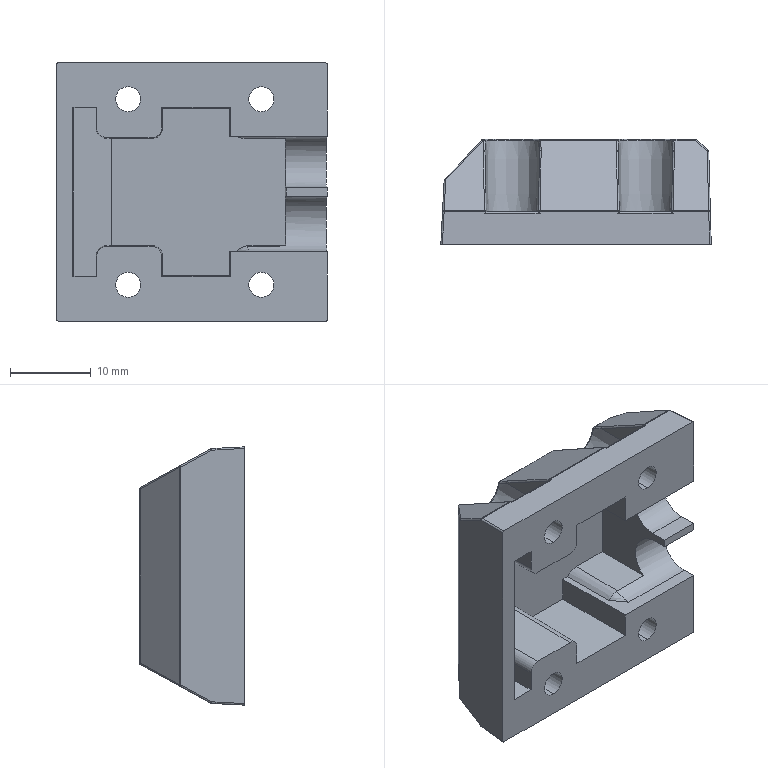Part | SolidWorks | features BaseBody 1 | 1 solid | 173 faces | box 33.5 x 13 x 32 mm | volume 5786 mm3 | cylinder 62 | plane 49 | spline 30 | sphere 18 | torus 8 | cone 6 | commonest cylinder face diameters 0.4 x42 3.1 x8 0.6 x6 2.4 x4 6.4 x1 6.9 x1